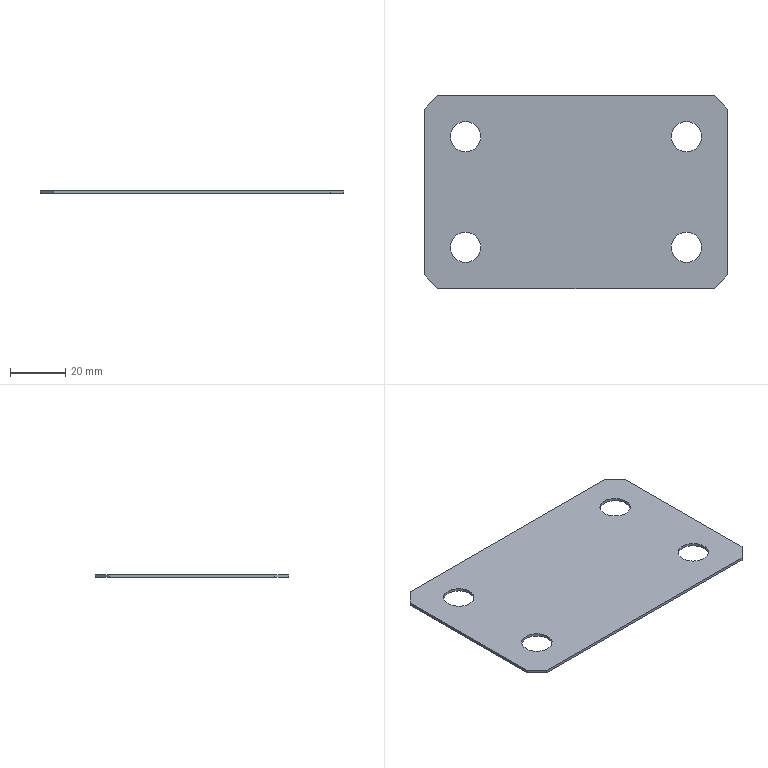Part | SolidWorks | features Chamfer 1, Extrusion 1, ICE 1 | 1 solid | 18 faces | box 110 x 70 x 1 mm | volume 7270 mm3 | plane 10 | cylinder 8 | commonest cylinder face diameters 11 x8
STEP:
#1=CARTESIAN_POINT('',(34.5,20.,0.));
#2=VERTEX_POINT('',#1);
#3=CARTESIAN_POINT('',(45.5,20.,0.));
#4=VERTEX_POINT('',#3);
#5=CARTESIAN_POINT('',(40.,20.,0.));
#6=DIRECTION('',(0.,0.,1.));
#7=DIRECTION('',(1.,0.,0.));
#8=AXIS2_PLACEMENT_3D('',#5,#6,#7);
#9=CIRCLE('',#8,5.5);
#10=EDGE_CURVE('',#2,#4,#9,.T.);
#11=ORIENTED_EDGE('',*,*,#10,.F.);
#12=CARTESIAN_POINT('',(34.5,20.,1.));
#13=VERTEX_POINT('',#12);
#14=CARTESIAN_POINT('',(34.5,20.,0.));
#15=DIRECTION('',(0.,0.,1.));
#16=VECTOR('',#15,1000.);
#17=LINE('',#14,#16);
#18=EDGE_CURVE('',#2,#13,#17,.T.);
#19=ORIENTED_EDGE('',*,*,#18,.T.);
#20=CARTESIAN_POINT('',(45.5,20.,1.));
#21=VERTEX_POINT('',#20);
#22=CARTESIAN_POINT('',(40.,20.,1.));
#23=DIRECTION('',(0.,0.,1.));
#24=DIRECTION('',(1.,0.,0.));
#25=AXIS2_PLACEMENT_3D('',#22,#23,#24);
#26=CIRCLE('',#25,5.5);
#27=EDGE_CURVE('',#13,#21,#26,.T.);
#28=ORIENTED_EDGE('',*,*,#27,.T.);
#29=CARTESIAN_POINT('',(45.5,20.,0.));
#30=DIRECTION('',(0.,0.,1.));
#31=VECTOR('',#30,1000.);
#32=LINE('',#29,#31);
#33=EDGE_CURVE('',#4,#21,#32,.T.);
#34=ORIENTED_EDGE('',*,*,#33,.F.);
#35=EDGE_LOOP('',(#11,#19,#28,#34));
#36=FACE_OUTER_BOUND('',#35,.T.);
#37=CARTESIAN_POINT('',(40.,20.,0.));
#38=DIRECTION('',(0.,0.,1.));
#39=DIRECTION('',(1.,0.,0.));
#40=AXIS2_PLACEMENT_3D('',#37,#38,#39);
#41=CYLINDRICAL_SURFACE('',#40,5.5);
#42=ADVANCED_FACE('',(#36),#41,.F.);
#43=CARTESIAN_POINT('',(-45.5,-20.,0.));
#44=VERTEX_POINT('',#43);
#45=CARTESIAN_POINT('',(-34.5,-20.,0.));
#46=VERTEX_POINT('',#45);
#47=CARTESIAN_POINT('',(-40.,-20.,0.));
#48=DIRECTION('',(0.,0.,1.));
#49=DIRECTION('',(1.,0.,0.));
#50=AXIS2_PLACEMENT_3D('',#47,#48,#49);
#51=CIRCLE('',#50,5.5);
#52=EDGE_CURVE('',#44,#46,#51,.T.);
#53=ORIENTED_EDGE('',*,*,#52,.F.);
#54=CARTESIAN_POINT('',(-45.5,-20.,1.));
#55=VERTEX_POINT('',#54);
#56=CARTESIAN_POINT('',(-45.5,-20.,0.));
#57=DIRECTION('',(0.,0.,1.));
#58=VECTOR('',#57,1000.);
#59=LINE('',#56,#58);
#60=EDGE_CURVE('',#44,#55,#59,.T.);
#61=ORIENTED_EDGE('',*,*,#60,.T.);
#62=CARTESIAN_POINT('',(-34.5,-20.,1.));
#63=VERTEX_POINT('',#62);
#64=CARTESIAN_POINT('',(-40.,-20.,1.));
#65=DIRECTION('',(0.,0.,1.));
#66=DIRECTION('',(1.,0.,0.));
#67=AXIS2_PLACEMENT_3D('',#64,#65,#66);
#68=CIRCLE('',#67,5.5);
#69=EDGE_CURVE('',#55,#63,#68,.T.);
#70=ORIENTED_EDGE('',*,*,#69,.T.);
#71=CARTESIAN_POINT('',(-34.5,-20.,0.));
#72=DIRECTION('',(0.,0.,1.));
#73=VECTOR('',#72,1000.);
#74=LINE('',#71,#73);
#75=EDGE_CURVE('',#46,#63,#74,.T.);
#76=ORIENTED_EDGE('',*,*,#75,.F.);
#77=EDGE_LOOP('',(#53,#61,#70,#76));
#78=FACE_OUTER_BOUND('',#77,.T.);
#79=CARTESIAN_POINT('',(-40.,-20.,0.));
#80=DIRECTION('',(0.,0.,1.));
#81=DIRECTION('',(1.,0.,0.));
#82=AXIS2_PLACEMENT_3D('',#79,#80,#81);
#83=CYLINDRICAL_SURFACE('',#82,5.5);
#84=ADVANCED_FACE('',(#78),#83,.F.);
#85=CARTESIAN_POINT('',(34.5,-20.,0.));
#86=VERTEX_POINT('',#85);
#87=CARTESIAN_POINT('',(45.5,-20.,0.));
#88=VERTEX_POINT('',#87);
#89=CARTESIAN_POINT('',(40.,-20.,0.));
#90=DIRECTION('',(0.,0.,1.));
#91=DIRECTION('',(1.,0.,0.));
#92=AXIS2_PLACEMENT_3D('',#89,#90,#91);
#93=CIRCLE('',#92,5.5);
#94=EDGE_CURVE('',#86,#88,#93,.T.);
#95=ORIENTED_EDGE('',*,*,#94,.F.);
#96=CARTESIAN_POINT('',(34.5,-20.,1.));
#97=VERTEX_POINT('',#96);
#98=CARTESIAN_POINT('',(34.5,-20.,0.));
#99=DIRECTION('',(0.,0.,1.));
#100=VECTOR('',#99,1000.);
#101=LINE('',#98,#100);
#102=EDGE_CURVE('',#86,#97,#101,.T.);
#103=ORIENTED_EDGE('',*,*,#102,.T.);
#104=CARTESIAN_POINT('',(45.5,-20.,1.));
#105=VERTEX_POINT('',#104);
#106=CARTESIAN_POINT('',(40.,-20.,1.));
#107=DIRECTION('',(0.,0.,1.));
#108=DIRECTION('',(1.,0.,0.));
#109=AXIS2_PLACEMENT_3D('',#106,#107,#108);
#110=CIRCLE('',#109,5.5);
#111=EDGE_CURVE('',#97,#105,#110,.T.);
#112=ORIENTED_EDGE('',*,*,#111,.T.);
#113=CARTESIAN_POINT('',(45.5,-20.,0.));
#114=DIRECTION('',(0.,0.,1.));
#115=VECTOR('',#114,1000.);
#116=LINE('',#113,#115);
#117=EDGE_CURVE('',#88,#105,#116,.T.);
#118=ORIENTED_EDGE('',*,*,#117,.F.);
#119=EDGE_LOOP('',(#95,#103,#112,#118));
#120=FACE_OUTER_BOUND('',#119,.T.);
#121=CARTESIAN_POINT('',(40.,-20.,0.));
#122=DIRECTION('',(0.,0.,1.));
#123=DIRECTION('',(1.,0.,0.));
#124=AXIS2_PLACEMENT_3D('',#121,#122,#123);
#125=CYLINDRICAL_SURFACE('',#124,5.5);
#126=ADVANCED_FACE('',(#120),#125,.F.);
#127=CARTESIAN_POINT('',(-45.5,20.,0.));
#128=VERTEX_POINT('',#127);
#129=CARTESIAN_POINT('',(-34.5,20.,0.));
#130=VERTEX_POINT('',#129);
#131=CARTESIAN_POINT('',(-40.,20.,0.));
#132=DIRECTION('',(0.,0.,1.));
#133=DIRECTION('',(1.,0.,0.));
#134=AXIS2_PLACEMENT_3D('',#131,#132,#133);
#135=CIRCLE('',#134,5.5);
#136=EDGE_CURVE('',#128,#130,#135,.T.);
#137=ORIENTED_EDGE('',*,*,#136,.F.);
#138=CARTESIAN_POINT('',(-45.5,20.,1.));
#139=VERTEX_POINT('',#138);
#140=CARTESIAN_POINT('',(-45.5,20.,0.));
#141=DIRECTION('',(0.,0.,1.));
#142=VECTOR('',#141,1000.);
#143=LINE('',#140,#142);
#144=EDGE_CURVE('',#128,#139,#143,.T.);
#145=ORIENTED_EDGE('',*,*,#144,.T.);
#146=CARTESIAN_POINT('',(-34.5,20.,1.));
#147=VERTEX_POINT('',#146);
#148=CARTESIAN_POINT('',(-40.,20.,1.));
#149=DIRECTION('',(0.,0.,1.));
#150=DIRECTION('',(1.,0.,0.));
#151=AXIS2_PLACEMENT_3D('',#148,#149,#150);
#152=CIRCLE('',#151,5.5);
#153=EDGE_CURVE('',#139,#147,#152,.T.);
#154=ORIENTED_EDGE('',*,*,#153,.T.);
#155=CARTESIAN_POINT('',(-34.5,20.,0.));
#156=DIRECTION('',(0.,0.,1.));
#157=VECTOR('',#156,1000.);
#158=LINE('',#155,#157);
#159=EDGE_CURVE('',#130,#147,#158,.T.);
#160=ORIENTED_EDGE('',*,*,#159,.F.);
#161=EDGE_LOOP('',(#137,#145,#154,#160));
#162=FACE_OUTER_BOUND('',#161,.T.);
#163=CARTESIAN_POINT('',(-40.,20.,0.));
#164=DIRECTION('',(0.,0.,1.));
#165=DIRECTION('',(1.,0.,0.));
#166=AXIS2_PLACEMENT_3D('',#163,#164,#165);
#167=CYLINDRICAL_SURFACE('',#166,5.5);
#168=ADVANCED_FACE('',(#162),#167,.F.);
#169=CARTESIAN_POINT('',(-55.,30.,0.));
#170=VERTEX_POINT('',#169);
#171=CARTESIAN_POINT('',(-55.,-30.,0.));
#172=VERTEX_POINT('',#171);
#173=CARTESIAN_POINT('',(-55.,35.,0.));
#174=DIRECTION('',(0.,-1.,0.));
#175=VECTOR('',#174,1000.);
#176=LINE('',#173,#175);
#177=EDGE_CURVE('',#170,#172,#176,.T.);
#178=ORIENTED_EDGE('',*,*,#177,.T.);
#179=CARTESIAN_POINT('',(-55.,-30.,1.));
#180=VERTEX_POINT('',#179);
#181=CARTESIAN_POINT('',(-55.,-30.,1.));
#182=DIRECTION('',(0.,0.,1.));
#183=VECTOR('',#182,1000.);
#184=LINE('',#181,#183);
#185=EDGE_CURVE('',#172,#180,#184,.T.);
#186=ORIENTED_EDGE('',*,*,#185,.T.);
#187=CARTESIAN_POINT('',(-55.,30.,1.));
#188=VERTEX_POINT('',#187);
#189=CARTESIAN_POINT('',(-55.,35.,1.));
#190=DIRECTION('',(0.,-1.,0.));
#191=VECTOR('',#190,1000.);
#192=LINE('',#189,#191);
#193=EDGE_CURVE('',#188,#180,#192,.T.);
#194=ORIENTED_EDGE('',*,*,#193,.F.);
#195=CARTESIAN_POINT('',(-55.,30.,1.));
#196=DIRECTION('',(0.,0.,-1.));
#197=VECTOR('',#196,1000.);
#198=LINE('',#195,#197);
#199=EDGE_CURVE('',#188,#170,#198,.T.);
#200=ORIENTED_EDGE('',*,*,#199,.T.);
#201=EDGE_LOOP('',(#178,#186,#194,#200));
#202=FACE_OUTER_BOUND('',#201,.T.);
#203=CARTESIAN_POINT('',(-55.,35.,1.));
#204=DIRECTION('',(1.,0.,0.));
#205=DIRECTION('',(0.,1.,0.));
#206=AXIS2_PLACEMENT_3D('',#203,#204,#205);
#207=PLANE('',#206);
#208=ADVANCED_FACE('',(#202),#207,.F.);
#209=CARTESIAN_POINT('',(-50.,-35.,1.));
#210=VERTEX_POINT('',#209);
#211=CARTESIAN_POINT('',(50.,-35.,1.));
#212=VERTEX_POINT('',#211);
#213=CARTESIAN_POINT('',(55.,-35.,1.));
#214=DIRECTION('',(1.,0.,0.));
#215=VECTOR('',#214,1000.);
#216=LINE('',#213,#215);
#217=EDGE_CURVE('',#210,#212,#216,.T.);
#218=ORIENTED_EDGE('',*,*,#217,.F.);
#219=CARTESIAN_POINT('',(-50.,-35.,0.));
#220=VERTEX_POINT('',#219);
#221=CARTESIAN_POINT('',(-50.,-35.,1.));
#222=DIRECTION('',(0.,0.,-1.));
#223=VECTOR('',#222,1000.);
#224=LINE('',#221,#223);
#225=EDGE_CURVE('',#210,#220,#224,.T.);
#226=ORIENTED_EDGE('',*,*,#225,.T.);
#227=CARTESIAN_POINT('',(50.,-35.,0.));
#228=VERTEX_POINT('',#227);
#229=CARTESIAN_POINT('',(55.,-35.,0.));
#230=DIRECTION('',(1.,0.,0.));
#231=VECTOR('',#230,1000.);
#232=LINE('',#229,#231);
#233=EDGE_CURVE('',#220,#228,#232,.T.);
#234=ORIENTED_EDGE('',*,*,#233,.T.);
#235=CARTESIAN_POINT('',(50.,-35.,1.));
#236=DIRECTION('',(0.,0.,1.));
#237=VECTOR('',#236,1000.);
#238=LINE('',#235,#237);
#239=EDGE_CURVE('',#228,#212,#238,.T.);
#240=ORIENTED_EDGE('',*,*,#239,.T.);
#241=EDGE_LOOP('',(#218,#226,#234,#240));
#242=FACE_OUTER_BOUND('',#241,.T.);
#243=CARTESIAN_POINT('',(55.,-35.,1.));
#244=DIRECTION('',(0.,1.,0.));
#245=DIRECTION('',(-1.,0.,0.));
#246=AXIS2_PLACEMENT_3D('',#243,#244,#245);
#247=PLANE('',#246);
#248=ADVANCED_FACE('',(#242),#247,.F.);
#249=CARTESIAN_POINT('',(55.,-30.,1.));
#250=VERTEX_POINT('',#249);
#251=CARTESIAN_POINT('',(55.,30.,1.));
#252=VERTEX_POINT('',#251);
#253=CARTESIAN_POINT('',(55.,35.,1.));
#254=DIRECTION('',(0.,1.,0.));
#255=VECTOR('',#254,1000.);
#256=LINE('',#253,#255);
#257=EDGE_CURVE('',#250,#252,#256,.T.);
#258=ORIENTED_EDGE('',*,*,#257,.F.);
#259=CARTESIAN_POINT('',(55.,-30.,0.));
#260=VERTEX_POINT('',#259);
#261=CARTESIAN_POINT('',(55.,-30.,1.));
#262=DIRECTION('',(0.,0.,-1.));
#263=VECTOR('',#262,1000.);
#264=LINE('',#261,#263);
#265=EDGE_CURVE('',#250,#260,#264,.T.);
#266=ORIENTED_EDGE('',*,*,#265,.T.);
#267=CARTESIAN_POINT('',(55.,30.,0.));
#268=VERTEX_POINT('',#267);
#269=CARTESIAN_POINT('',(55.,35.,0.));
#270=DIRECTION('',(0.,1.,0.));
#271=VECTOR('',#270,1000.);
#272=LINE('',#269,#271);
#273=EDGE_CURVE('',#260,#268,#272,.T.);
#274=ORIENTED_EDGE('',*,*,#273,.T.);
#275=CARTESIAN_POINT('',(55.,30.,1.));
#276=DIRECTION('',(0.,0.,1.));
#277=VECTOR('',#276,1000.);
#278=LINE('',#275,#277);
#279=EDGE_CURVE('',#268,#252,#278,.T.);
#280=ORIENTED_EDGE('',*,*,#279,.T.);
#281=EDGE_LOOP('',(#258,#266,#274,#280));
#282=FACE_OUTER_BOUND('',#281,.T.);
#283=CARTESIAN_POINT('',(55.,35.,1.));
#284=DIRECTION('',(-1.,0.,0.));
#285=DIRECTION('',(0.,-1.,0.));
#286=AXIS2_PLACEMENT_3D('',#283,#284,#285);
#287=PLANE('',#286);
#288=ADVANCED_FACE('',(#282),#287,.F.);
#289=CARTESIAN_POINT('',(50.,35.,1.));
#290=VERTEX_POINT('',#289);
#291=CARTESIAN_POINT('',(-50.,35.,1.));
#292=VERTEX_POINT('',#291);
#293=CARTESIAN_POINT('',(55.,35.,1.));
#294=DIRECTION('',(-1.,0.,0.));
#295=VECTOR('',#294,1000.);
#296=LINE('',#293,#295);
#297=EDGE_CURVE('',#290,#292,#296,.T.);
#298=ORIENTED_EDGE('',*,*,#297,.F.);
#299=CARTESIAN_POINT('',(50.,35.,0.));
#300=VERTEX_POINT('',#299);
#301=CARTESIAN_POINT('',(50.,35.,1.));
#302=DIRECTION('',(0.,0.,-1.));
#303=VECTOR('',#302,1000.);
#304=LINE('',#301,#303);
#305=EDGE_CURVE('',#290,#300,#304,.T.);
#306=ORIENTED_EDGE('',*,*,#305,.T.);
#307=CARTESIAN_POINT('',(-50.,35.,0.));
#308=VERTEX_POINT('',#307);
#309=CARTESIAN_POINT('',(55.,35.,0.));
#310=DIRECTION('',(-1.,0.,0.));
#311=VECTOR('',#310,1000.);
#312=LINE('',#309,#311);
#313=EDGE_CURVE('',#300,#308,#312,.T.);
#314=ORIENTED_EDGE('',*,*,#313,.T.);
#315=CARTESIAN_POINT('',(-50.,35.,1.));
#316=DIRECTION('',(0.,0.,1.));
#317=VECTOR('',#316,1000.);
#318=LINE('',#315,#317);
#319=EDGE_CURVE('',#308,#292,#318,.T.);
#320=ORIENTED_EDGE('',*,*,#319,.T.);
#321=EDGE_LOOP('',(#298,#306,#314,#320));
#322=FACE_OUTER_BOUND('',#321,.T.);
#323=CARTESIAN_POINT('',(55.,35.,1.));
#324=DIRECTION('',(0.,-1.,0.));
#325=DIRECTION('',(1.,0.,0.));
#326=AXIS2_PLACEMENT_3D('',#323,#324,#325);
#327=PLANE('',#326);
#328=ADVANCED_FACE('',(#322),#327,.F.);
#329=CARTESIAN_POINT('',(40.,20.,1.));
#330=DIRECTION('',(0.,0.,1.));
#331=DIRECTION('',(1.,0.,0.));
#332=AXIS2_PLACEMENT_3D('',#329,#330,#331);
#333=CIRCLE('',#332,5.5);
#334=EDGE_CURVE('',#21,#13,#333,.T.);
#335=ORIENTED_EDGE('',*,*,#334,.F.);
#336=ORIENTED_EDGE('',*,*,#27,.F.);
#337=EDGE_LOOP('',(#335,#336));
#338=FACE_BOUND('',#337,.T.);
#339=CARTESIAN_POINT('',(-40.,-20.,1.));
#340=DIRECTION('',(0.,0.,1.));
#341=DIRECTION('',(1.,0.,0.));
#342=AXIS2_PLACEMENT_3D('',#339,#340,#341);
#343=CIRCLE('',#342,5.5);
#344=EDGE_CURVE('',#63,#55,#343,.T.);
#345=ORIENTED_EDGE('',*,*,#344,.F.);
#346=ORIENTED_EDGE('',*,*,#69,.F.);
#347=EDGE_LOOP('',(#345,#346));
#348=FACE_BOUND('',#347,.T.);
#349=CARTESIAN_POINT('',(40.,-20.,1.));
#350=DIRECTION('',(0.,0.,1.));
#351=DIRECTION('',(1.,0.,0.));
#352=AXIS2_PLACEMENT_3D('',#349,#350,#351);
#353=CIRCLE('',#352,5.5);
#354=EDGE_CURVE('',#105,#97,#353,.T.);
#355=ORIENTED_EDGE('',*,*,#354,.F.);
#356=ORIENTED_EDGE('',*,*,#111,.F.);
#357=EDGE_LOOP('',(#355,#356));
#358=FACE_BOUND('',#357,.T.);
#359=CARTESIAN_POINT('',(-40.,20.,1.));
#360=DIRECTION('',(0.,0.,1.));
#361=DIRECTION('',(1.,0.,0.));
#362=AXIS2_PLACEMENT_3D('',#359,#360,#361);
#363=CIRCLE('',#362,5.5);
#364=EDGE_CURVE('',#147,#139,#363,.T.);
#365=ORIENTED_EDGE('',*,*,#364,.F.);
#366=ORIENTED_EDGE('',*,*,#153,.F.);
#367=EDGE_LOOP('',(#365,#366));
#368=FACE_BOUND('',#367,.T.);
#369=ORIENTED_EDGE('',*,*,#193,.T.);
#370=CARTESIAN_POINT('',(-50.,-35.,1.));
#371=DIRECTION('',(0.7071,-0.7071,0.));
#372=VECTOR('',#371,1000.);
#373=LINE('',#370,#372);
#374=EDGE_CURVE('',#180,#210,#373,.T.);
#375=ORIENTED_EDGE('',*,*,#374,.T.);
#376=ORIENTED_EDGE('',*,*,#217,.T.);
#377=CARTESIAN_POINT('',(55.,-30.,1.));
#378=DIRECTION('',(0.7071,0.7071,0.));
#379=VECTOR('',#378,1000.);
#380=LINE('',#377,#379);
#381=EDGE_CURVE('',#212,#250,#380,.T.);
#382=ORIENTED_EDGE('',*,*,#381,.T.);
#383=ORIENTED_EDGE('',*,*,#257,.T.);
#384=CARTESIAN_POINT('',(50.,35.,1.));
#385=DIRECTION('',(-0.7071,0.7071,0.));
#386=VECTOR('',#385,1000.);
#387=LINE('',#384,#386);
#388=EDGE_CURVE('',#252,#290,#387,.T.);
#389=ORIENTED_EDGE('',*,*,#388,.T.);
#390=ORIENTED_EDGE('',*,*,#297,.T.);
#391=CARTESIAN_POINT('',(-55.,30.,1.));
#392=DIRECTION('',(-0.7071,-0.7071,0.));
#393=VECTOR('',#392,1000.);
#394=LINE('',#391,#393);
#395=EDGE_CURVE('',#292,#188,#394,.T.);
#396=ORIENTED_EDGE('',*,*,#395,.T.);
#397=EDGE_LOOP('',(#369,#375,#376,#382,#383,#389,#390,#396));
#398=FACE_OUTER_BOUND('',#397,.T.);
#399=CARTESIAN_POINT('',(0.,0.,1.));
#400=DIRECTION('',(0.,0.,-1.));
#401=DIRECTION('',(-1.,0.,0.));
#402=AXIS2_PLACEMENT_3D('',#399,#400,#401);
#403=PLANE('',#402);
#404=ADVANCED_FACE('',(#338,#348,#358,#368,#398),#403,.F.);
#405=CARTESIAN_POINT('',(40.,20.,0.));
#406=DIRECTION('',(0.,0.,1.));
#407=DIRECTION('',(1.,0.,0.));
#408=AXIS2_PLACEMENT_3D('',#405,#406,#407);
#409=CIRCLE('',#408,5.5);
#410=EDGE_CURVE('',#4,#2,#409,.T.);
#411=ORIENTED_EDGE('',*,*,#410,.T.);
#412=ORIENTED_EDGE('',*,*,#10,.T.);
#413=EDGE_LOOP('',(#411,#412));
#414=FACE_BOUND('',#413,.T.);
#415=CARTESIAN_POINT('',(-40.,-20.,0.));
#416=DIRECTION('',(0.,0.,1.));
#417=DIRECTION('',(1.,0.,0.));
#418=AXIS2_PLACEMENT_3D('',#415,#416,#417);
#419=CIRCLE('',#418,5.5);
#420=EDGE_CURVE('',#46,#44,#419,.T.);
#421=ORIENTED_EDGE('',*,*,#420,.T.);
#422=ORIENTED_EDGE('',*,*,#52,.T.);
#423=EDGE_LOOP('',(#421,#422));
#424=FACE_BOUND('',#423,.T.);
#425=CARTESIAN_POINT('',(40.,-20.,0.));
#426=DIRECTION('',(0.,0.,1.));
#427=DIRECTION('',(1.,0.,0.));
#428=AXIS2_PLACEMENT_3D('',#425,#426,#427);
#429=CIRCLE('',#428,5.5);
#430=EDGE_CURVE('',#88,#86,#429,.T.);
#431=ORIENTED_EDGE('',*,*,#430,.T.);
#432=ORIENTED_EDGE('',*,*,#94,.T.);
#433=EDGE_LOOP('',(#431,#432));
#434=FACE_BOUND('',#433,.T.);
#435=CARTESIAN_POINT('',(-40.,20.,0.));
#436=DIRECTION('',(0.,0.,1.));
#437=DIRECTION('',(1.,0.,0.));
#438=AXIS2_PLACEMENT_3D('',#435,#436,#437);
#439=CIRCLE('',#438,5.5);
#440=EDGE_CURVE('',#130,#128,#439,.T.);
#441=ORIENTED_EDGE('',*,*,#440,.T.);
#442=ORIENTED_EDGE('',*,*,#136,.T.);
#443=EDGE_LOOP('',(#441,#442));
#444=FACE_BOUND('',#443,.T.);
#445=ORIENTED_EDGE('',*,*,#233,.F.);
#446=CARTESIAN_POINT('',(-42.5,-42.5,0.));
#447=DIRECTION('',(-0.7071,0.7071,0.));
#448=VECTOR('',#447,1000.);
#449=LINE('',#446,#448);
#450=EDGE_CURVE('',#220,#172,#449,.T.);
#451=ORIENTED_EDGE('',*,*,#450,.T.);
#452=ORIENTED_EDGE('',*,*,#177,.F.);
#453=CARTESIAN_POINT('',(-42.5,42.5,0.));
#454=DIRECTION('',(0.7071,0.7071,0.));
#455=VECTOR('',#454,1000.);
#456=LINE('',#453,#455);
#457=EDGE_CURVE('',#170,#308,#456,.T.);
#458=ORIENTED_EDGE('',*,*,#457,.T.);
#459=ORIENTED_EDGE('',*,*,#313,.F.);
#460=CARTESIAN_POINT('',(42.5,42.5,0.));
#461=DIRECTION('',(0.7071,-0.7071,0.));
#462=VECTOR('',#461,1000.);
#463=LINE('',#460,#462);
#464=EDGE_CURVE('',#300,#268,#463,.T.);
#465=ORIENTED_EDGE('',*,*,#464,.T.);
#466=ORIENTED_EDGE('',*,*,#273,.F.);
#467=CARTESIAN_POINT('',(42.5,-42.5,0.));
#468=DIRECTION('',(-0.7071,-0.7071,0.));
#469=VECTOR('',#468,1000.);
#470=LINE('',#467,#469);
#471=EDGE_CURVE('',#260,#228,#470,.T.);
#472=ORIENTED_EDGE('',*,*,#471,.T.);
#473=EDGE_LOOP('',(#445,#451,#452,#458,#459,#465,#466,#472));
#474=FACE_OUTER_BOUND('',#473,.T.);
#475=CARTESIAN_POINT('',(0.,0.,0.));
#476=DIRECTION('',(0.,0.,-1.));
#477=DIRECTION('',(-1.,0.,0.));
#478=AXIS2_PLACEMENT_3D('',#475,#476,#477);
#479=PLANE('',#478);
#480=ADVANCED_FACE('',(#414,#424,#434,#444,#474),#479,.T.);
#481=ORIENTED_EDGE('',*,*,#144,.F.);
#482=ORIENTED_EDGE('',*,*,#440,.F.);
#483=ORIENTED_EDGE('',*,*,#159,.T.);
#484=ORIENTED_EDGE('',*,*,#364,.T.);
#485=EDGE_LOOP('',(#481,#482,#483,#484));
#486=FACE_OUTER_BOUND('',#485,.T.);
#487=CARTESIAN_POINT('',(-40.,20.,0.));
#488=DIRECTION('',(0.,0.,1.));
#489=DIRECTION('',(1.,0.,0.));
#490=AXIS2_PLACEMENT_3D('',#487,#488,#489);
#491=CYLINDRICAL_SURFACE('',#490,5.5);
#492=ADVANCED_FACE('',(#486),#491,.F.);
#493=ORIENTED_EDGE('',*,*,#102,.F.);
#494=ORIENTED_EDGE('',*,*,#430,.F.);
#495=ORIENTED_EDGE('',*,*,#117,.T.);
#496=ORIENTED_EDGE('',*,*,#354,.T.);
#497=EDGE_LOOP('',(#493,#494,#495,#496));
#498=FACE_OUTER_BOUND('',#497,.T.);
#499=CARTESIAN_POINT('',(40.,-20.,0.));
#500=DIRECTION('',(0.,0.,1.));
#501=DIRECTION('',(1.,0.,0.));
#502=AXIS2_PLACEMENT_3D('',#499,#500,#501);
#503=CYLINDRICAL_SURFACE('',#502,5.5);
#504=ADVANCED_FACE('',(#498),#503,.F.);
#505=ORIENTED_EDGE('',*,*,#60,.F.);
#506=ORIENTED_EDGE('',*,*,#420,.F.);
#507=ORIENTED_EDGE('',*,*,#75,.T.);
#508=ORIENTED_EDGE('',*,*,#344,.T.);
#509=EDGE_LOOP('',(#505,#506,#507,#508));
#510=FACE_OUTER_BOUND('',#509,.T.);
#511=CARTESIAN_POINT('',(-40.,-20.,0.));
#512=DIRECTION('',(0.,0.,1.));
#513=DIRECTION('',(1.,0.,0.));
#514=AXIS2_PLACEMENT_3D('',#511,#512,#513);
#515=CYLINDRICAL_SURFACE('',#514,5.5);
#516=ADVANCED_FACE('',(#510),#515,.F.);
#517=ORIENTED_EDGE('',*,*,#18,.F.);
#518=ORIENTED_EDGE('',*,*,#410,.F.);
#519=ORIENTED_EDGE('',*,*,#33,.T.);
#520=ORIENTED_EDGE('',*,*,#334,.T.);
#521=EDGE_LOOP('',(#517,#518,#519,#520));
#522=FACE_OUTER_BOUND('',#521,.T.);
#523=CARTESIAN_POINT('',(40.,20.,0.));
#524=DIRECTION('',(0.,0.,1.));
#525=DIRECTION('',(1.,0.,0.));
#526=AXIS2_PLACEMENT_3D('',#523,#524,#525);
#527=CYLINDRICAL_SURFACE('',#526,5.5);
#528=ADVANCED_FACE('',(#522),#527,.F.);
#529=ORIENTED_EDGE('',*,*,#374,.F.);
#530=ORIENTED_EDGE('',*,*,#185,.F.);
#531=ORIENTED_EDGE('',*,*,#450,.F.);
#532=ORIENTED_EDGE('',*,*,#225,.F.);
#533=EDGE_LOOP('',(#529,#530,#531,#532));
#534=FACE_OUTER_BOUND('',#533,.T.);
#535=CARTESIAN_POINT('',(-50.,-35.,1.));
#536=DIRECTION('',(0.7071,0.7071,0.));
#537=DIRECTION('',(0.,0.,-1.));
#538=AXIS2_PLACEMENT_3D('',#535,#536,#537);
#539=PLANE('',#538);
#540=ADVANCED_FACE('',(#534),#539,.F.);
#541=ORIENTED_EDGE('',*,*,#381,.F.);
#542=ORIENTED_EDGE('',*,*,#239,.F.);
#543=ORIENTED_EDGE('',*,*,#471,.F.);
#544=ORIENTED_EDGE('',*,*,#265,.F.);
#545=EDGE_LOOP('',(#541,#542,#543,#544));
#546=FACE_OUTER_BOUND('',#545,.T.);
#547=CARTESIAN_POINT('',(55.,-30.,1.));
#548=DIRECTION('',(-0.7071,0.7071,0.));
#549=DIRECTION('',(0.,0.,-1.));
#550=AXIS2_PLACEMENT_3D('',#547,#548,#549);
#551=PLANE('',#550);
#552=ADVANCED_FACE('',(#546),#551,.F.);
#553=ORIENTED_EDGE('',*,*,#388,.F.);
#554=ORIENTED_EDGE('',*,*,#279,.F.);
#555=ORIENTED_EDGE('',*,*,#464,.F.);
#556=ORIENTED_EDGE('',*,*,#305,.F.);
#557=EDGE_LOOP('',(#553,#554,#555,#556));
#558=FACE_OUTER_BOUND('',#557,.T.);
#559=CARTESIAN_POINT('',(50.,35.,1.));
#560=DIRECTION('',(-0.7071,-0.7071,0.));
#561=DIRECTION('',(0.,0.,-1.));
#562=AXIS2_PLACEMENT_3D('',#559,#560,#561);
#563=PLANE('',#562);
#564=ADVANCED_FACE('',(#558),#563,.F.);
#565=ORIENTED_EDGE('',*,*,#395,.F.);
#566=ORIENTED_EDGE('',*,*,#319,.F.);
#567=ORIENTED_EDGE('',*,*,#457,.F.);
#568=ORIENTED_EDGE('',*,*,#199,.F.);
#569=EDGE_LOOP('',(#565,#566,#567,#568));
#570=FACE_OUTER_BOUND('',#569,.T.);
#571=CARTESIAN_POINT('',(-55.,30.,1.));
#572=DIRECTION('',(0.7071,-0.7071,0.));
#573=DIRECTION('',(0.,0.,-1.));
#574=AXIS2_PLACEMENT_3D('',#571,#572,#573);
#575=PLANE('',#574);
#576=ADVANCED_FACE('',(#570),#575,.F.);
#577=CLOSED_SHELL('',(#42,#84,#126,#168,#208,#248,#288,#328,#404,#480,#492,#504,#516,#528,#540,#552,#564,#576));
#578=MANIFOLD_SOLID_BREP('',#577);
#579=CARTESIAN_POINT('',(0.,0.,0.));
#580=DIRECTION('',(0.,0.,1.));
#581=DIRECTION('',(1.,0.,0.));
#582=AXIS2_PLACEMENT_3D('',#579,#580,#581);
#583=(LENGTH_UNIT()NAMED_UNIT(*)SI_UNIT(.MILLI.,.METRE.));
#584=UNCERTAINTY_MEASURE_WITH_UNIT(LENGTH_MEASURE(0.00001),#583,'','');
#585=(NAMED_UNIT(*)PLANE_ANGLE_UNIT()SI_UNIT($,.RADIAN.));
#586=(NAMED_UNIT(*)SI_UNIT($,.STERADIAN.)SOLID_ANGLE_UNIT());
#587=(GEOMETRIC_REPRESENTATION_CONTEXT(3)GLOBAL_UNCERTAINTY_ASSIGNED_CONTEXT((#584))GLOBAL_UNIT_ASSIGNED_CONTEXT((#583,#585,#586))REPRESENTATION_CONTEXT('',''));
#588=ADVANCED_BREP_SHAPE_REPRESENTATION('',(#578,#582),#587);